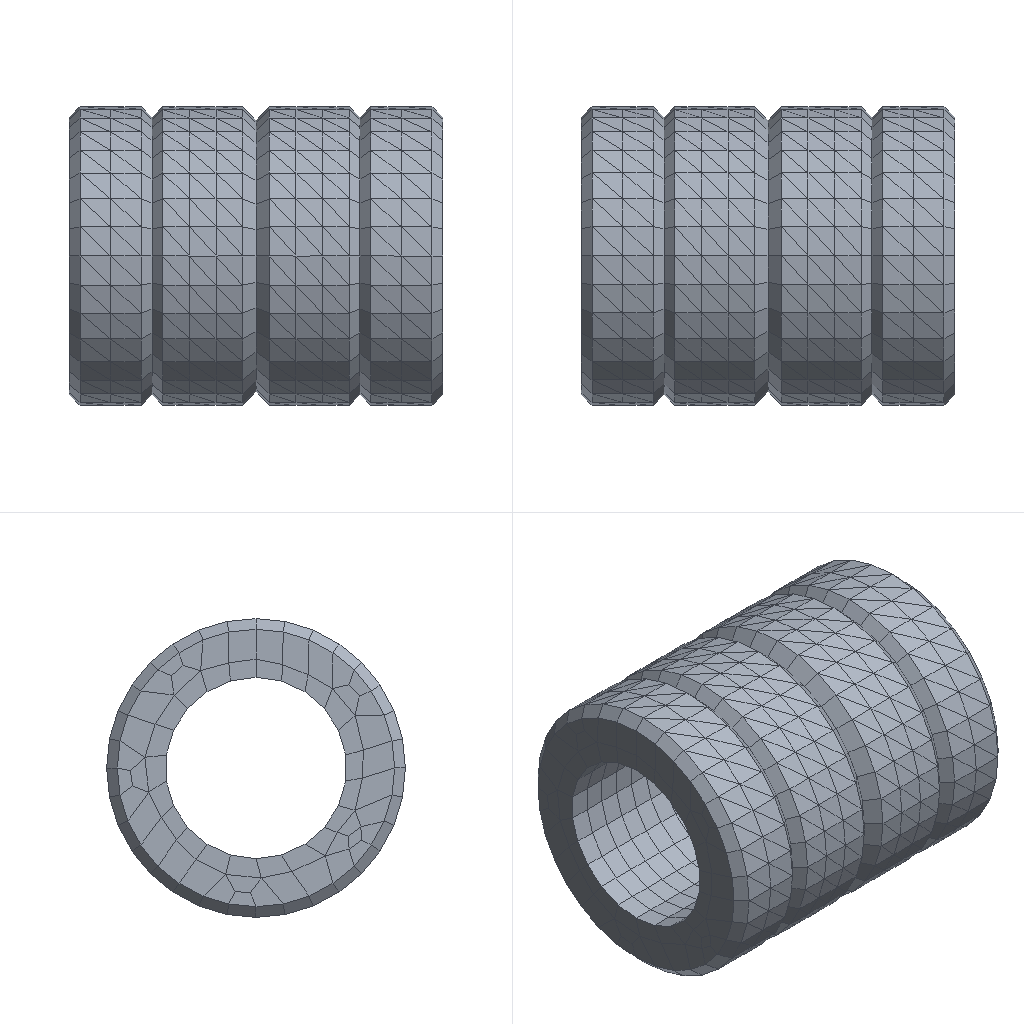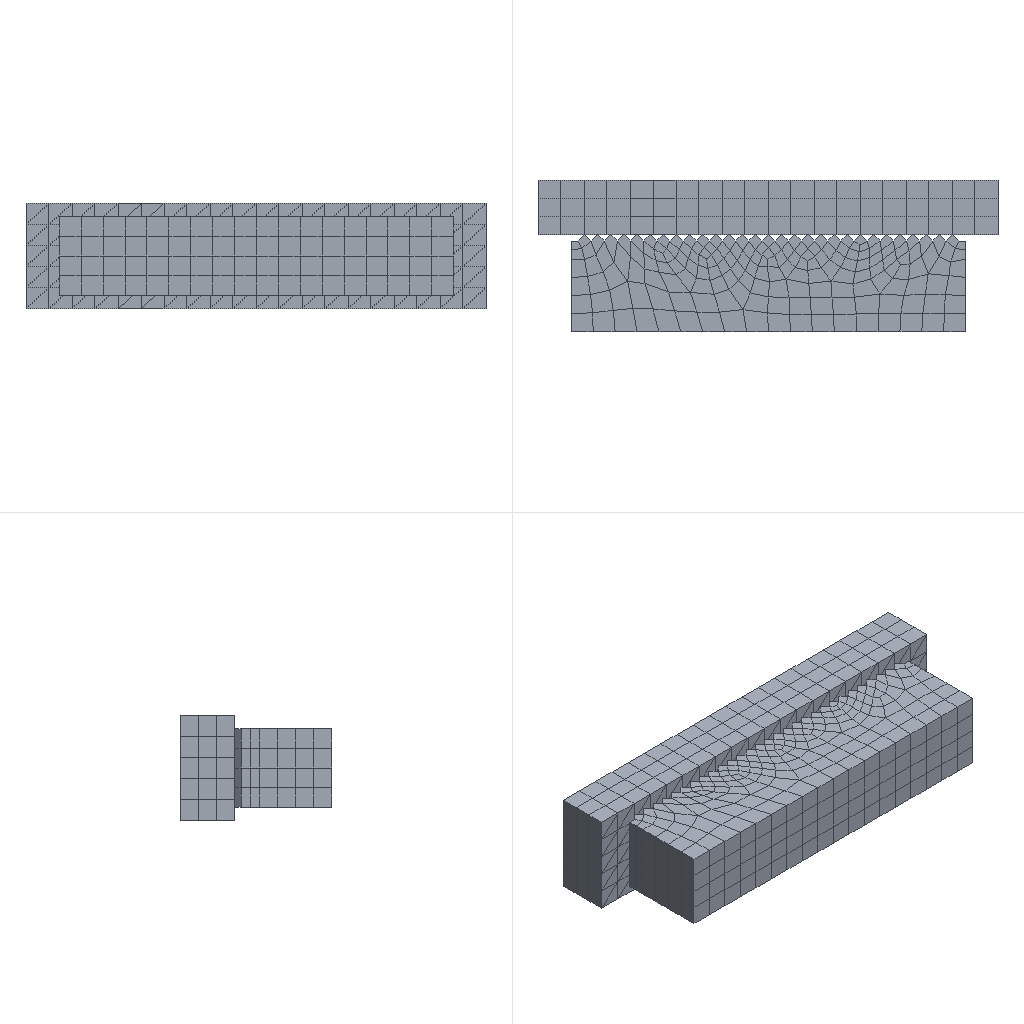Simulation study | ansys workbench
Set-up summary:
category,name,step,type,value,unit,region
solver,ansys_mapdl
solver,version,,,22.1
solver,version,,,22.1
units,MPA,,stated
analysis,deck1,,static,static
load_step,requested,,,1
analysis,nlgeom,,,False
mesh,nodes,,,5708
mesh,elements,,,1416
element_type,ANSYS 186 (type 1),,solid,692
element_type,ANSYS 186 (type 2),,solid,300
element_type,ANSYS 174 (type 3),,contact,124
element_type,ANSYS 170 (type 4),,target,124
element_type,ANSYS 154 (type 5),,surface,76
element_type,ANSYS 154 (type 6),,surface,100
load,load commands in deck,,count,6
bc,support commands in deck,,count,1
named_set,_FIXEDSU,,component
analysis,deck2,,static,static
load_step,requested,,,1
analysis,nlgeom,,,False
mesh,nodes,,,6088
mesh,elements,,,1418
element_type,ANSYS 186 (type 1),,solid,1098
element_type,ANSYS 174 (type 2),,contact,320
element_type,ANSYS 170 (type 3),,target,0
load,load commands in deck,,count,3
bc,support commands in deck,,count,1
named_set,_FIXEDSU,,component
material,1,,in results
material,2,,in results
material,1,,in results
check,setup vs results,,match,176 surface effect element(s) are not in the reader's mesh and were not compared
check,setup vs results,,match,results also hold 0 node(s) and 1 element(s) the deck makes with ['EN']; those were not compared; 1 node(s) the solver created internally for pilot nodes (ansys-fenxi-3/胶桶有限元分析/fenc_files/dp0/SYS/MECH/solve.out) are in the results only
Results summary:
result,analysis,,,static
result,last_loadstep,,,1
result,primary field,,,displacement
result,reaction total,1,FX,85000.0,N
result,reaction total,1,FY,-780.0,N
result,reaction total,1,FZ,-0.0,N
result,mass,,,1.9e-05,"NMM: mm, ton, N, s, mV, mA, degC"
result,analysis,,,static
result,last_loadstep,,,1
result,primary field,,,displacement
result,reaction total,1,FX,-0.0,N
result,reaction total,1,FY,0.0,N
result,reaction total,1,FZ,-0.0,N
result,mass,,,0.000833,"NMM: mm, ton, N, s, mV, mA, degC"